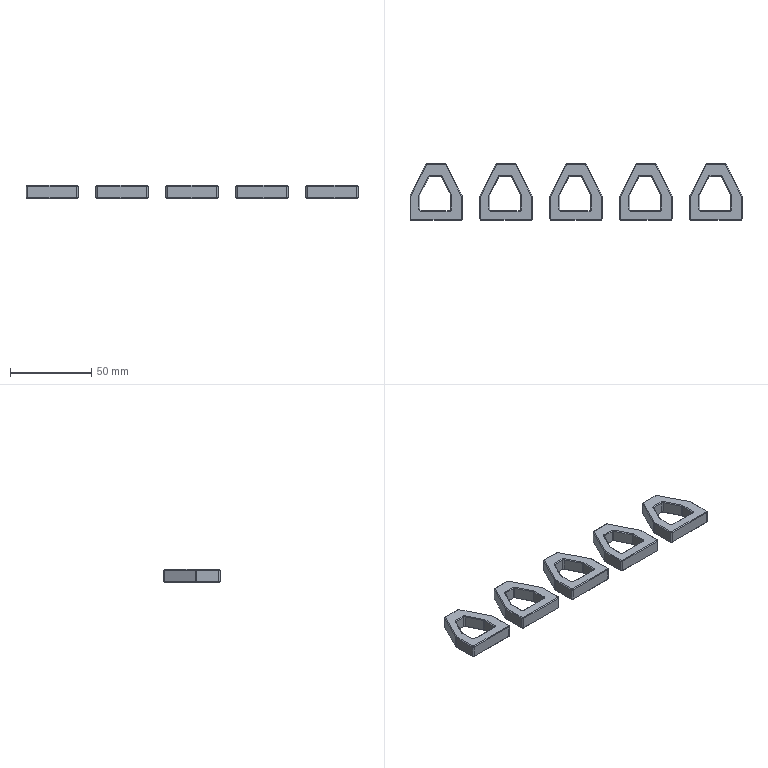NC program | NX | posted with a generic post | part box 204 x 35 x 8 mm
Lines 19 to 965 of 15564:
(ZLEVEL_PROFILE_COPY_1 , TOOL : D10)
N36 T15 M6
N38 G54
N40 G17 G0 G90 X4.326 Y-1.972 S9500 M3
N42 G43 Z30. H15
N44 Z1.5
N46 G94 G1 X1.14 Y4.4 Z1.127 F1000.
N48 X-0.14 Z1.06
N50 X-3.9 Y-3.12 Z0.619
N52 Y-6.4 Z0.447
N54 X4.9 Z-0.014
N56 Y-3.12 Z-0.186
N58 X1.14 Y4.4 Z-0.627
N60 X-0.14 Z-0.694
N62 X-2.753 Y-0.827 Z-1.
N64 X-3.9 Y-3.12 F3500.
N66 Y-6.4
N68 X4.9
N70 Y-3.12
N72 X1.14 Y4.4
N74 X-0.14
N76 X-2.753 Y-0.827
N78 X-3.9 Y-3.12 Z-1.077
N80 Y-6.4 Z-1.175
N82 X4.9 Z-1.438
N84 Y-3.12 Z-1.536
N86 X1.14 Y4.4 Z-1.787
N88 X-0.14 Z-1.825
N90 X-2.753 Y-0.827 Z-2.
N92 X-3.9 Y-3.12 Z-2.077
N94 Y-6.4 Z-2.175
N96 X4.9 Z-2.438
N98 Y-3.12 Z-2.536
N100 X1.14 Y4.4 Z-2.787
N102 X-0.14 Z-2.825
N104 X-2.753 Y-0.827 Z-3.
N106 X-3.9 Y-3.12 Z-3.077
N108 Y-6.4 Z-3.175
N110 X4.9 Z-3.438
N112 Y-3.12 Z-3.536
N114 X1.14 Y4.4 Z-3.787
N116 X-0.14 Z-3.825
N118 X-2.753 Y-0.827 Z-4.
N120 X-3.9 Y-3.12 Z-4.077
N122 Y-6.4 Z-4.175
N124 X4.9 Z-4.438
N126 Y-3.12 Z-4.536
N128 X1.14 Y4.4 Z-4.787
N130 X-0.14 Z-4.825
N132 X-2.753 Y-0.827 Z-5.
N134 X-3.9 Y-3.12 Z-5.077
N136 Y-6.4 Z-5.175
N138 X4.9 Z-5.438
N140 Y-3.12 Z-5.536
N142 X1.14 Y4.4 Z-5.787
N144 X-0.14 Z-5.825
N146 X-2.753 Y-0.827 Z-6.
N148 X-3.9 Y-3.12 Z-6.077
N150 Y-6.4 Z-6.175
N152 X4.9 Z-6.438
N154 Y-3.12 Z-6.536
N156 X1.14 Y4.4 Z-6.787
N158 X-0.14 Z-6.825
N160 X-2.753 Y-0.827 Z-7.
N162 X-3.9 Y-3.12 Z-7.077
N164 Y-6.4 Z-7.175
N166 X4.9 Z-7.438
N168 Y-3.12 Z-7.536
N170 X1.14 Y4.4 Z-7.787
N172 X-0.14 Z-7.825
N174 X-2.753 Y-0.827 Z-8.
N176 X-3.9 Y-3.12
N178 Y-6.4
N180 X4.9
N182 Y-3.12
N184 X1.14 Y4.4
N186 X-0.14
N188 X-2.753 Y-0.827
N190 Z-6.5
N192 G0 Z53.
N194 X-46.504 Y-6.4
N196 Z1.5
N198 G1 X-38.1 Z1.06 F1000.
N200 Y-3.12 Z0.888
N202 X-41.86 Y4.4 Z0.447
N204 X-43.14 Z0.38
N206 X-46.9 Y-3.12 Z-0.061
N208 Y-6.4 Z-0.233
N210 X-38.1 Z-0.694
N212 Y-3.12 Z-0.866
N214 X-39.247 Y-0.827 Z-1.
N216 X-41.86 Y4.4 F3500.
N218 X-43.14
N220 X-46.9 Y-3.12
N222 Y-6.4
N224 X-38.1
N226 Y-3.12
N228 X-39.247 Y-0.827
N230 X-41.86 Y4.4 Z-1.175
N232 X-43.14 Z-1.213
N234 X-46.9 Y-3.12 Z-1.464
N236 Y-6.4 Z-1.562
N238 X-38.1 Z-1.825
N240 Y-3.12 Z-1.923
N242 X-39.247 Y-0.827 Z-2.
N244 X-41.86 Y4.4 Z-2.175
N246 X-43.14 Z-2.213
N248 X-46.9 Y-3.12 Z-2.464
N250 Y-6.4 Z-2.562
N252 X-38.1 Z-2.825
N254 Y-3.12 Z-2.923
N256 X-39.247 Y-0.827 Z-3.
N258 X-41.86 Y4.4 Z-3.175
N260 X-43.14 Z-3.213
N262 X-46.9 Y-3.12 Z-3.464
N264 Y-6.4 Z-3.562
N266 X-38.1 Z-3.825
N268 Y-3.12 Z-3.923
N270 X-39.247 Y-0.827 Z-4.
N272 X-41.86 Y4.4 Z-4.175
N274 X-43.14 Z-4.213
N276 X-46.9 Y-3.12 Z-4.464
N278 Y-6.4 Z-4.562
N280 X-38.1 Z-4.825
N282 Y-3.12 Z-4.923
N284 X-39.247 Y-0.827 Z-5.
N286 X-41.86 Y4.4 Z-5.175
N288 X-43.14 Z-5.213
N290 X-46.9 Y-3.12 Z-5.464
N292 Y-6.4 Z-5.562
N294 X-38.1 Z-5.825
N296 Y-3.12 Z-5.923
N298 X-39.247 Y-0.827 Z-6.
N300 X-41.86 Y4.4 Z-6.175
N302 X-43.14 Z-6.213
N304 X-46.9 Y-3.12 Z-6.464
N306 Y-6.4 Z-6.562
N308 X-38.1 Z-6.825
N310 Y-3.12 Z-6.923
N312 X-39.247 Y-0.827 Z-7.
N314 X-41.86 Y4.4 Z-7.175
N316 X-43.14 Z-7.213
N318 X-46.9 Y-3.12 Z-7.464
N320 Y-6.4 Z-7.562
N322 X-38.1 Z-7.825
N324 Y-3.12 Z-7.923
N326 X-39.247 Y-0.827 Z-8.
N328 X-41.86 Y4.4
N330 X-43.14
N332 X-46.9 Y-3.12
N334 Y-6.4
N336 X-38.1
N338 Y-3.12
N340 X-39.247 Y-0.827
N342 Z-6.5
N344 G0 Z53.
N346 X-81.674 Y-1.972
N348 Z1.5
N350 G1 X-84.86 Y4.4 Z1.127 F1000.
N352 X-86.14 Z1.06
N354 X-89.9 Y-3.12 Z0.619
N356 Y-6.4 Z0.447
N358 X-81.1 Z-0.014
N360 Y-3.12 Z-0.186
N362 X-84.86 Y4.4 Z-0.627
N364 X-86.14 Z-0.694
N366 X-88.753 Y-0.827 Z-1.
N368 X-89.9 Y-3.12 F3500.
N370 Y-6.4
N372 X-81.1
N374 Y-3.12
N376 X-84.86 Y4.4
N378 X-86.14
N380 X-88.753 Y-0.827
N382 X-89.9 Y-3.12 Z-1.077
N384 Y-6.4 Z-1.175
N386 X-81.1 Z-1.438
N388 Y-3.12 Z-1.536
N390 X-84.86 Y4.4 Z-1.787
N392 X-86.14 Z-1.825
N394 X-88.753 Y-0.827 Z-2.
N396 X-89.9 Y-3.12 Z-2.077
N398 Y-6.4 Z-2.175
N400 X-81.1 Z-2.438
N402 Y-3.12 Z-2.536
N404 X-84.86 Y4.4 Z-2.787
N406 X-86.14 Z-2.825
N408 X-88.753 Y-0.827 Z-3.
N410 X-89.9 Y-3.12 Z-3.077
N412 Y-6.4 Z-3.175
N414 X-81.1 Z-3.438
N416 Y-3.12 Z-3.536
N418 X-84.86 Y4.4 Z-3.787
N420 X-86.14 Z-3.825
N422 X-88.753 Y-0.827 Z-4.
N424 X-89.9 Y-3.12 Z-4.077
N426 Y-6.4 Z-4.175
N428 X-81.1 Z-4.438
N430 Y-3.12 Z-4.536
N432 X-84.86 Y4.4 Z-4.787
N434 X-86.14 Z-4.825
N436 X-88.753 Y-0.827 Z-5.
N438 X-89.9 Y-3.12 Z-5.077
N440 Y-6.4 Z-5.175
N442 X-81.1 Z-5.438
N444 Y-3.12 Z-5.536
N446 X-84.86 Y4.4 Z-5.787
N448 X-86.14 Z-5.825
N450 X-88.753 Y-0.827 Z-6.
N452 X-89.9 Y-3.12 Z-6.077
N454 Y-6.4 Z-6.175
N456 X-81.1 Z-6.438
N458 Y-3.12 Z-6.536
N460 X-84.86 Y4.4 Z-6.787
N462 X-86.14 Z-6.825
N464 X-88.753 Y-0.827 Z-7.
N466 X-89.9 Y-3.12 Z-7.077
N468 Y-6.4 Z-7.175
N470 X-81.1 Z-7.438
N472 Y-3.12 Z-7.536
N474 X-84.86 Y4.4 Z-7.787
N476 X-86.14 Z-7.825
N478 X-88.753 Y-0.827 Z-8.
N480 X-89.9 Y-3.12
N482 Y-6.4
N484 X-81.1
N486 Y-3.12
N488 X-84.86 Y4.4
N490 X-86.14
N492 X-88.753 Y-0.827
N494 Z-6.5
N496 G0 Z53.
N498 X82.496 Y-6.4
N500 Z1.5
N502 G1 X90.9 Z1.06 F1000.
N504 Y-3.12 Z0.888
N506 X87.14 Y4.4 Z0.447
N508 X85.86 Z0.38
N510 X82.1 Y-3.12 Z-0.061
N512 Y-6.4 Z-0.233
N514 X90.9 Z-0.694
N516 Y-3.12 Z-0.866
N518 X89.753 Y-0.827 Z-1.
N520 X87.14 Y4.4 F3500.
N522 X85.86
N524 X82.1 Y-3.12
N526 Y-6.4
N528 X90.9
N530 Y-3.12
N532 X89.753 Y-0.827
N534 X87.14 Y4.4 Z-1.175
N536 X85.86 Z-1.213
N538 X82.1 Y-3.12 Z-1.464
N540 Y-6.4 Z-1.562
N542 X90.9 Z-1.825
N544 Y-3.12 Z-1.923
N546 X89.753 Y-0.827 Z-2.
N548 X87.14 Y4.4 Z-2.175
N550 X85.86 Z-2.213
N552 X82.1 Y-3.12 Z-2.464
N554 Y-6.4 Z-2.562
N556 X90.9 Z-2.825
N558 Y-3.12 Z-2.923
N560 X89.753 Y-0.827 Z-3.
N562 X87.14 Y4.4 Z-3.175
N564 X85.86 Z-3.213
N566 X82.1 Y-3.12 Z-3.464
N568 Y-6.4 Z-3.562
N570 X90.9 Z-3.825
N572 Y-3.12 Z-3.923
N574 X89.753 Y-0.827 Z-4.
N576 X87.14 Y4.4 Z-4.175
N578 X85.86 Z-4.213
N580 X82.1 Y-3.12 Z-4.464
N582 Y-6.4 Z-4.562
N584 X90.9 Z-4.825
N586 Y-3.12 Z-4.923
N588 X89.753 Y-0.827 Z-5.
N590 X87.14 Y4.4 Z-5.175
N592 X85.86 Z-5.213
N594 X82.1 Y-3.12 Z-5.464
N596 Y-6.4 Z-5.562
N598 X90.9 Z-5.825
N600 Y-3.12 Z-5.923
N602 X89.753 Y-0.827 Z-6.
N604 X87.14 Y4.4 Z-6.175
N606 X85.86 Z-6.213
N608 X82.1 Y-3.12 Z-6.464
N610 Y-6.4 Z-6.562
N612 X90.9 Z-6.825
N614 Y-3.12 Z-6.923
N616 X89.753 Y-0.827 Z-7.
N618 X87.14 Y4.4 Z-7.175
N620 X85.86 Z-7.213
N622 X82.1 Y-3.12 Z-7.464
N624 Y-6.4 Z-7.562
N626 X90.9 Z-7.825
N628 Y-3.12 Z-7.923
N630 X89.753 Y-0.827 Z-8.
N632 X87.14 Y4.4
N634 X85.86
N636 X82.1 Y-3.12
N638 Y-6.4
N640 X90.9
N642 Y-3.12
N644 X89.753 Y-0.827
N646 Z-6.5
N648 G0 Z53.
N650 X39.496 Y-6.4
N652 Z1.5
N654 G1 X47.9 Z1.06 F1000.
N656 Y-3.12 Z0.888
N658 X44.14 Y4.4 Z0.447
N660 X42.86 Z0.38
N662 X39.1 Y-3.12 Z-0.061
N664 Y-6.4 Z-0.233
N666 X47.9 Z-0.694
N668 Y-3.12 Z-0.866
N670 X46.753 Y-0.827 Z-1.
N672 X44.14 Y4.4 F3500.
N674 X42.86
N676 X39.1 Y-3.12
N678 Y-6.4
N680 X47.9
N682 Y-3.12
N684 X46.753 Y-0.827
N686 X44.14 Y4.4 Z-1.175
N688 X42.86 Z-1.213
N690 X39.1 Y-3.12 Z-1.464
N692 Y-6.4 Z-1.562
N694 X47.9 Z-1.825
N696 Y-3.12 Z-1.923
N698 X46.753 Y-0.827 Z-2.
N700 X44.14 Y4.4 Z-2.175
N702 X42.86 Z-2.213
N704 X39.1 Y-3.12 Z-2.464
N706 Y-6.4 Z-2.562
N708 X47.9 Z-2.825
N710 Y-3.12 Z-2.923
N712 X46.753 Y-0.827 Z-3.
N714 X44.14 Y4.4 Z-3.175
N716 X42.86 Z-3.213
N718 X39.1 Y-3.12 Z-3.464
N720 Y-6.4 Z-3.562
N722 X47.9 Z-3.825
N724 Y-3.12 Z-3.923
N726 X46.753 Y-0.827 Z-4.
N728 X44.14 Y4.4 Z-4.175
N730 X42.86 Z-4.213
N732 X39.1 Y-3.12 Z-4.464
N734 Y-6.4 Z-4.562
N736 X47.9 Z-4.825
N738 Y-3.12 Z-4.923
N740 X46.753 Y-0.827 Z-5.
N742 X44.14 Y4.4 Z-5.175
N744 X42.86 Z-5.213
N746 X39.1 Y-3.12 Z-5.464
N748 Y-6.4 Z-5.562
N750 X47.9 Z-5.825
N752 Y-3.12 Z-5.923
N754 X46.753 Y-0.827 Z-6.
N756 X44.14 Y4.4 Z-6.175
N758 X42.86 Z-6.213
N760 X39.1 Y-3.12 Z-6.464
N762 Y-6.4 Z-6.562
N764 X47.9 Z-6.825
N766 Y-3.12 Z-6.923
N768 X46.753 Y-0.827 Z-7.
N770 X44.14 Y4.4 Z-7.175
N772 X42.86 Z-7.213
N774 X39.1 Y-3.12 Z-7.464
N776 Y-6.4 Z-7.562
N778 X47.9 Z-7.825
N780 Y-3.12 Z-7.923
N782 X46.753 Y-0.827 Z-8.
N784 X44.14 Y4.4
N786 X42.86
N788 X39.1 Y-3.12
N790 Y-6.4
N792 X47.9
N794 Y-3.12
N796 X46.753 Y-0.827
N798 Z-6.5
N800 G0 Z53.
N802 X60.548 Y5.808
N804 Z1.5
N806 G1 X63.727 Y-0.55 Z1.127 F1000.
N808 X64.1 Y-2.13 Z1.042
N810 Y-17.106 Z0.258
N812 X63.707 Y-18.737 Z0.17
N814 X62.887 Y-20.201 Z0.082
N816 X61.701 Y-21.387 Z-0.006
N818 X60.237 Y-22.207 Z-0.094
N820 X58.606 Y-22.6 Z-0.182
N822 X43. Z-1.
N824 X28. F3500.
N826 G2 X21.9 Y-16.5 R6.1
N828 G1 Y-2.736
N830 G2 X22.544 Y-0.008 R6.1
N832 G1 X32.162 Y19.228
N834 G2 X37.618 Y22.6 R6.1
N836 G1 X48.382
N838 G2 X53.838 Y19.228 R6.1
N840 G1 X63.456 Y-0.008
N842 G2 X64.1 Y-2.736 R6.1
N844 G1 Y-16.5
N846 G2 X58. Y-22.6 R6.1
N848 G1 X43.
N850 X28. Z-1.1
N852 X27.402 Y-22.571 Z-1.104
N854 X26.81 Y-22.483 Z-1.108
N856 X26.229 Y-22.337 Z-1.112
N858 X25.666 Y-22.136 Z-1.116
N860 X25.124 Y-21.88 Z-1.12
N862 X24.611 Y-21.572 Z-1.124
N864 X24.13 Y-21.215 Z-1.128
N866 X23.687 Y-20.813 Z-1.132
N868 X23.285 Y-20.37 Z-1.136
N870 X22.928 Y-19.889 Z-1.14
N872 X22.62 Y-19.376 Z-1.144
N874 X22.364 Y-18.834 Z-1.148
N876 X22.163 Y-18.271 Z-1.152
N878 X22.017 Y-17.69 Z-1.156
N880 X21.929 Y-17.098 Z-1.16
N882 X21.9 Y-16.5 Z-1.164
N884 Y-2.736 Z-1.256
N886 X21.918 Y-2.265 Z-1.259
N888 X21.973 Y-1.797 Z-1.263
N890 X22.063 Y-1.335 Z-1.266
N892 X22.189 Y-0.88 Z-1.269
N894 X22.35 Y-0.437 Z-1.272
N896 X22.544 Y-0.008 Z-1.275
N898 X32.162 Y19.228 Z-1.419
N900 X32.437 Y19.719 Z-1.423
N902 X32.755 Y20.183 Z-1.426
N904 X33.115 Y20.615 Z-1.43
N906 X33.513 Y21.012 Z-1.434
N908 X33.947 Y21.371 Z-1.438
N910 X34.411 Y21.689 Z-1.441
N912 X34.903 Y21.962 Z-1.445
N914 X35.418 Y22.189 Z-1.449
N916 X35.951 Y22.368 Z-1.453
N918 X36.499 Y22.496 Z-1.457
N920 X37.056 Y22.574 Z-1.46
N922 X37.618 Y22.6 Z-1.464
N924 X48.382 Z-1.536
N926 X48.944 Y22.574 Z-1.54
N928 X49.501 Y22.496 Z-1.543
N930 X50.049 Y22.368 Z-1.547
N932 X50.582 Y22.189 Z-1.551
N934 X51.097 Y21.962 Z-1.555
N936 X51.589 Y21.689 Z-1.559
N938 X52.053 Y21.371 Z-1.562
N940 X52.487 Y21.012 Z-1.566
N942 X52.885 Y20.615 Z-1.57
N944 X53.245 Y20.183 Z-1.574
N946 X53.563 Y19.719 Z-1.577
N948 X53.838 Y19.228 Z-1.581
N950 X63.456 Y-0.008 Z-1.725
N952 X63.65 Y-0.437 Z-1.728
N954 X63.811 Y-0.88 Z-1.731
N956 X63.937 Y-1.335 Z-1.734
N958 X64.027 Y-1.797 Z-1.737
N960 X64.082 Y-2.265 Z-1.741
N962 X64.1 Y-2.736 Z-1.744
N964 Y-16.5 Z-1.836
N966 X64.071 Y-17.098 Z-1.84
N968 X63.983 Y-17.69 Z-1.844
N970 X63.837 Y-18.271 Z-1.848
N972 X63.636 Y-18.834 Z-1.852
N974 X63.38 Y-19.376 Z-1.856
N976 X63.072 Y-19.889 Z-1.86
N978 X62.715 Y-20.37 Z-1.864
N980 X62.313 Y-20.813 Z-1.868
N982 X61.87 Y-21.215 Z-1.872
N984 X61.389 Y-21.572 Z-1.876
N986 X60.876 Y-21.88 Z-1.88
N988 X60.334 Y-22.136 Z-1.884
N990 X59.771 Y-22.337 Z-1.888
N992 X59.19 Y-22.483 Z-1.892
N994 X58.598 Y-22.571 Z-1.896
N996 X58. Y-22.6 Z-1.9
N998 X43. Z-2.
N1000 X28. Z-2.1
N1002 X27.402 Y-22.571 Z-2.104
N1004 X26.81 Y-22.483 Z-2.108
N1006 X26.229 Y-22.337 Z-2.112
N1008 X25.666 Y-22.136 Z-2.116
N1010 X25.124 Y-21.88 Z-2.12
N1012 X24.611 Y-21.572 Z-2.124
N1014 X24.13 Y-21.215 Z-2.128
N1016 X23.687 Y-20.813 Z-2.132
N1018 X23.285 Y-20.37 Z-2.136
N1020 X22.928 Y-19.889 Z-2.14
N1022 X22.62 Y-19.376 Z-2.144
N1024 X22.364 Y-18.834 Z-2.148
N1026 X22.163 Y-18.271 Z-2.152
N1028 X22.017 Y-17.69 Z-2.156
N1030 X21.929 Y-17.098 Z-2.16
N1032 X21.9 Y-16.5 Z-2.164
N1034 Y-2.736 Z-2.256
N1036 X21.918 Y-2.265 Z-2.259
N1038 X21.973 Y-1.797 Z-2.263
N1040 X22.063 Y-1.335 Z-2.266
N1042 X22.189 Y-0.88 Z-2.269
N1044 X22.35 Y-0.437 Z-2.272
N1046 X22.544 Y-0.008 Z-2.275
N1048 X32.162 Y19.228 Z-2.419
N1050 X32.437 Y19.719 Z-2.423
N1052 X32.755 Y20.183 Z-2.426
N1054 X33.115 Y20.615 Z-2.43
N1056 X33.513 Y21.012 Z-2.434
N1058 X33.947 Y21.371 Z-2.438
N1060 X34.411 Y21.689 Z-2.441
N1062 X34.903 Y21.962 Z-2.445
N1064 X35.418 Y22.189 Z-2.449
N1066 X35.951 Y22.368 Z-2.453
N1068 X36.499 Y22.496 Z-2.457
N1070 X37.056 Y22.574 Z-2.46
N1072 X37.618 Y22.6 Z-2.464
N1074 X48.382 Z-2.536
N1076 X48.944 Y22.574 Z-2.54
N1078 X49.501 Y22.496 Z-2.543
N1080 X50.049 Y22.368 Z-2.547
N1082 X50.582 Y22.189 Z-2.551
N1084 X51.097 Y21.962 Z-2.555
N1086 X51.589 Y21.689 Z-2.559
N1088 X52.053 Y21.371 Z-2.562
N1090 X52.487 Y21.012 Z-2.566
N1092 X52.885 Y20.615 Z-2.57
N1094 X53.245 Y20.183 Z-2.574
N1096 X53.563 Y19.719 Z-2.577
N1098 X53.838 Y19.228 Z-2.581
N1100 X63.456 Y-0.008 Z-2.725
N1102 X63.65 Y-0.437 Z-2.728
N1104 X63.811 Y-0.88 Z-2.731
N1106 X63.937 Y-1.335 Z-2.734
N1108 X64.027 Y-1.797 Z-2.737
N1110 X64.082 Y-2.265 Z-2.741
N1112 X64.1 Y-2.736 Z-2.744
N1114 Y-16.5 Z-2.836
N1116 X64.071 Y-17.098 Z-2.84
N1118 X63.983 Y-17.69 Z-2.844
N1120 X63.837 Y-18.271 Z-2.848
N1122 X63.636 Y-18.834 Z-2.852
N1124 X63.38 Y-19.376 Z-2.856
N1126 X63.072 Y-19.889 Z-2.86
N1128 X62.715 Y-20.37 Z-2.864
N1130 X62.313 Y-20.813 Z-2.868
N1132 X61.87 Y-21.215 Z-2.872
N1134 X61.389 Y-21.572 Z-2.876
N1136 X60.876 Y-21.88 Z-2.88
N1138 X60.334 Y-22.136 Z-2.884
N1140 X59.771 Y-22.337 Z-2.888
N1142 X59.19 Y-22.483 Z-2.892
N1144 X58.598 Y-22.571 Z-2.896
N1146 X58. Y-22.6 Z-2.9
N1148 X43. Z-3.
N1150 X28. Z-3.1
N1152 X27.402 Y-22.571 Z-3.104
N1154 X26.81 Y-22.483 Z-3.108
N1156 X26.229 Y-22.337 Z-3.112
N1158 X25.666 Y-22.136 Z-3.116
N1160 X25.124 Y-21.88 Z-3.12
N1162 X24.611 Y-21.572 Z-3.124
N1164 X24.13 Y-21.215 Z-3.128
N1166 X23.687 Y-20.813 Z-3.132
N1168 X23.285 Y-20.37 Z-3.136
N1170 X22.928 Y-19.889 Z-3.14
N1172 X22.62 Y-19.376 Z-3.144
N1174 X22.364 Y-18.834 Z-3.148
N1176 X22.163 Y-18.271 Z-3.152
N1178 X22.017 Y-17.69 Z-3.156
N1180 X21.929 Y-17.098 Z-3.16
N1182 X21.9 Y-16.5 Z-3.164
N1184 Y-2.736 Z-3.256
N1186 X21.918 Y-2.265 Z-3.259
N1188 X21.973 Y-1.797 Z-3.263
N1190 X22.063 Y-1.335 Z-3.266
N1192 X22.189 Y-0.88 Z-3.269
N1194 X22.35 Y-0.437 Z-3.272
N1196 X22.544 Y-0.008 Z-3.275
N1198 X32.162 Y19.228 Z-3.419
N1200 X32.437 Y19.719 Z-3.423
N1202 X32.755 Y20.183 Z-3.426
N1204 X33.115 Y20.615 Z-3.43
N1206 X33.513 Y21.012 Z-3.434
N1208 X33.947 Y21.371 Z-3.438
N1210 X34.411 Y21.689 Z-3.441
N1212 X34.903 Y21.962 Z-3.445
N1214 X35.418 Y22.189 Z-3.449
N1216 X35.951 Y22.368 Z-3.453
N1218 X36.499 Y22.496 Z-3.457
N1220 X37.056 Y22.574 Z-3.46
N1222 X37.618 Y22.6 Z-3.464
N1224 X48.382 Z-3.536
N1226 X48.944 Y22.574 Z-3.54
N1228 X49.501 Y22.496 Z-3.543
N1230 X50.049 Y22.368 Z-3.547
N1232 X50.582 Y22.189 Z-3.551
N1234 X51.097 Y21.962 Z-3.555
N1236 X51.589 Y21.689 Z-3.559
N1238 X52.053 Y21.371 Z-3.562
N1240 X52.487 Y21.012 Z-3.566
N1242 X52.885 Y20.615 Z-3.57
N1244 X53.245 Y20.183 Z-3.574
N1246 X53.563 Y19.719 Z-3.577
N1248 X53.838 Y19.228 Z-3.581
N1250 X63.456 Y-0.008 Z-3.725
N1252 X63.65 Y-0.437 Z-3.728
N1254 X63.811 Y-0.88 Z-3.731
N1256 X63.937 Y-1.335 Z-3.734
N1258 X64.027 Y-1.797 Z-3.737
N1260 X64.082 Y-2.265 Z-3.741
N1262 X64.1 Y-2.736 Z-3.744
N1264 Y-16.5 Z-3.836
N1266 X64.071 Y-17.098 Z-3.84
N1268 X63.983 Y-17.69 Z-3.844
N1270 X63.837 Y-18.271 Z-3.848
N1272 X63.636 Y-18.834 Z-3.852
N1274 X63.38 Y-19.376 Z-3.856
N1276 X63.072 Y-19.889 Z-3.86
N1278 X62.715 Y-20.37 Z-3.864
N1280 X62.313 Y-20.813 Z-3.868
N1282 X61.87 Y-21.215 Z-3.872
N1284 X61.389 Y-21.572 Z-3.876
N1286 X60.876 Y-21.88 Z-3.88
N1288 X60.334 Y-22.136 Z-3.884
N1290 X59.771 Y-22.337 Z-3.888
N1292 X59.19 Y-22.483 Z-3.892
N1294 X58.598 Y-22.571 Z-3.896
N1296 X58. Y-22.6 Z-3.9
N1298 X43. Z-4.
N1300 X28. Z-4.1
N1302 X27.402 Y-22.571 Z-4.104
N1304 X26.81 Y-22.483 Z-4.108
N1306 X26.229 Y-22.337 Z-4.112
N1308 X25.666 Y-22.136 Z-4.116
N1310 X25.124 Y-21.88 Z-4.12
N1312 X24.611 Y-21.572 Z-4.124
N1314 X24.13 Y-21.215 Z-4.128
N1316 X23.687 Y-20.813 Z-4.132
N1318 X23.285 Y-20.37 Z-4.136
N1320 X22.928 Y-19.889 Z-4.14
N1322 X22.62 Y-19.376 Z-4.144
N1324 X22.364 Y-18.834 Z-4.148
N1326 X22.163 Y-18.271 Z-4.152
N1328 X22.017 Y-17.69 Z-4.156
N1330 X21.929 Y-17.098 Z-4.16
N1332 X21.9 Y-16.5 Z-4.164
N1334 Y-2.736 Z-4.256
N1336 X21.918 Y-2.265 Z-4.259
N1338 X21.973 Y-1.797 Z-4.263
N1340 X22.063 Y-1.335 Z-4.266
N1342 X22.189 Y-0.88 Z-4.269
N1344 X22.35 Y-0.437 Z-4.272
N1346 X22.544 Y-0.008 Z-4.275
N1348 X32.162 Y19.228 Z-4.419
N1350 X32.437 Y19.719 Z-4.423
N1352 X32.755 Y20.183 Z-4.426
N1354 X33.115 Y20.615 Z-4.43
N1356 X33.513 Y21.012 Z-4.434
N1358 X33.947 Y21.371 Z-4.438
N1360 X34.411 Y21.689 Z-4.441
N1362 X34.903 Y21.962 Z-4.445
N1364 X35.418 Y22.189 Z-4.449
N1366 X35.951 Y22.368 Z-4.453
N1368 X36.499 Y22.496 Z-4.457
N1370 X37.056 Y22.574 Z-4.46
N1372 X37.618 Y22.6 Z-4.464
N1374 X48.382 Z-4.536
N1376 X48.944 Y22.574 Z-4.54
N1378 X49.501 Y22.496 Z-4.543
N1380 X50.049 Y22.368 Z-4.547
N1382 X50.582 Y22.189 Z-4.551
N1384 X51.097 Y21.962 Z-4.555
N1386 X51.589 Y21.689 Z-4.559
N1388 X52.053 Y21.371 Z-4.562
N1390 X52.487 Y21.012 Z-4.566
N1392 X52.885 Y20.615 Z-4.57
N1394 X53.245 Y20.183 Z-4.574
N1396 X53.563 Y19.719 Z-4.577
N1398 X53.838 Y19.228 Z-4.581
N1400 X63.456 Y-0.008 Z-4.725
N1402 X63.65 Y-0.437 Z-4.728
N1404 X63.811 Y-0.88 Z-4.731
N1406 X63.937 Y-1.335 Z-4.734
N1408 X64.027 Y-1.797 Z-4.737
N1410 X64.082 Y-2.265 Z-4.741
N1412 X64.1 Y-2.736 Z-4.744
N1414 Y-16.5 Z-4.836
N1416 X64.071 Y-17.098 Z-4.84
N1418 X63.983 Y-17.69 Z-4.844
N1420 X63.837 Y-18.271 Z-4.848
N1422 X63.636 Y-18.834 Z-4.852
N1424 X63.38 Y-19.376 Z-4.856
N1426 X63.072 Y-19.889 Z-4.86
N1428 X62.715 Y-20.37 Z-4.864
N1430 X62.313 Y-20.813 Z-4.868
N1432 X61.87 Y-21.215 Z-4.872
N1434 X61.389 Y-21.572 Z-4.876
N1436 X60.876 Y-21.88 Z-4.88
N1438 X60.334 Y-22.136 Z-4.884
N1440 X59.771 Y-22.337 Z-4.888
N1442 X59.19 Y-22.483 Z-4.892
N1444 X58.598 Y-22.571 Z-4.896
N1446 X58. Y-22.6 Z-4.9
N1448 X43. Z-5.
N1450 X28. Z-5.1
N1452 X27.402 Y-22.571 Z-5.104
N1454 X26.81 Y-22.483 Z-5.108
N1456 X26.229 Y-22.337 Z-5.112
N1458 X25.666 Y-22.136 Z-5.116
N1460 X25.124 Y-21.88 Z-5.12
N1462 X24.611 Y-21.572 Z-5.124
N1464 X24.13 Y-21.215 Z-5.128
N1466 X23.687 Y-20.813 Z-5.132
N1468 X23.285 Y-20.37 Z-5.136
N1470 X22.928 Y-19.889 Z-5.14
N1472 X22.62 Y-19.376 Z-5.144
N1474 X22.364 Y-18.834 Z-5.148
N1476 X22.163 Y-18.271 Z-5.152
N1478 X22.017 Y-17.69 Z-5.156
N1480 X21.929 Y-17.098 Z-5.16
N1482 X21.9 Y-16.5 Z-5.164
N1484 Y-2.736 Z-5.256
N1486 X21.918 Y-2.265 Z-5.259
N1488 X21.973 Y-1.797 Z-5.263
N1490 X22.063 Y-1.335 Z-5.266
N1492 X22.189 Y-0.88 Z-5.269
N1494 X22.35 Y-0.437 Z-5.272
N1496 X22.544 Y-0.008 Z-5.275
N1498 X32.162 Y19.228 Z-5.419
N1500 X32.437 Y19.719 Z-5.423
N1502 X32.755 Y20.183 Z-5.426
N1504 X33.115 Y20.615 Z-5.43
N1506 X33.513 Y21.012 Z-5.434
N1508 X33.947 Y21.371 Z-5.438
N1510 X34.411 Y21.689 Z-5.441
N1512 X34.903 Y21.962 Z-5.445
N1514 X35.418 Y22.189 Z-5.449
N1516 X35.951 Y22.368 Z-5.453
N1518 X36.499 Y22.496 Z-5.457
N1520 X37.056 Y22.574 Z-5.46
N1522 X37.618 Y22.6 Z-5.464
N1524 X48.382 Z-5.536
N1526 X48.944 Y22.574 Z-5.54
N1528 X49.501 Y22.496 Z-5.543
N1530 X50.049 Y22.368 Z-5.547
N1532 X50.582 Y22.189 Z-5.551
N1534 X51.097 Y21.962 Z-5.555
N1536 X51.589 Y21.689 Z-5.559
N1538 X52.053 Y21.371 Z-5.562
N1540 X52.487 Y21.012 Z-5.566
N1542 X52.885 Y20.615 Z-5.57
N1544 X53.245 Y20.183 Z-5.574
N1546 X53.563 Y19.719 Z-5.577
N1548 X53.838 Y19.228 Z-5.581
N1550 X63.456 Y-0.008 Z-5.725
N1552 X63.65 Y-0.437 Z-5.728
N1554 X63.811 Y-0.88 Z-5.731
N1556 X63.937 Y-1.335 Z-5.734
N1558 X64.027 Y-1.797 Z-5.737
N1560 X64.082 Y-2.265 Z-5.741
N1562 X64.1 Y-2.736 Z-5.744
N1564 Y-16.5 Z-5.836
N1566 X64.071 Y-17.098 Z-5.84
N1568 X63.983 Y-17.69 Z-5.844
N1570 X63.837 Y-18.271 Z-5.848
N1572 X63.636 Y-18.834 Z-5.852
N1574 X63.38 Y-19.376 Z-5.856
N1576 X63.072 Y-19.889 Z-5.86
N1578 X62.715 Y-20.37 Z-5.864
N1580 X62.313 Y-20.813 Z-5.868
N1582 X61.87 Y-21.215 Z-5.872
N1584 X61.389 Y-21.572 Z-5.876
N1586 X60.876 Y-21.88 Z-5.88
N1588 X60.334 Y-22.136 Z-5.884
N1590 X59.771 Y-22.337 Z-5.888
N1592 X59.19 Y-22.483 Z-5.892
N1594 X58.598 Y-22.571 Z-5.896
N1596 X58. Y-22.6 Z-5.9
N1598 X43. Z-6.
N1600 X28. Z-6.1
N1602 X27.402 Y-22.571 Z-6.104
N1604 X26.81 Y-22.483 Z-6.108
N1606 X26.229 Y-22.337 Z-6.112
N1608 X25.666 Y-22.136 Z-6.116
N1610 X25.124 Y-21.88 Z-6.12
N1612 X24.611 Y-21.572 Z-6.124
N1614 X24.13 Y-21.215 Z-6.128
N1616 X23.687 Y-20.813 Z-6.132
N1618 X23.285 Y-20.37 Z-6.136
N1620 X22.928 Y-19.889 Z-6.14
N1622 X22.62 Y-19.376 Z-6.144
N1624 X22.364 Y-18.834 Z-6.148
N1626 X22.163 Y-18.271 Z-6.152
N1628 X22.017 Y-17.69 Z-6.156
N1630 X21.929 Y-17.098 Z-6.16
N1632 X21.9 Y-16.5 Z-6.164
N1634 Y-2.736 Z-6.256
N1636 X21.918 Y-2.265 Z-6.259
N1638 X21.973 Y-1.797 Z-6.263
N1640 X22.063 Y-1.335 Z-6.266
N1642 X22.189 Y-0.88 Z-6.269
N1644 X22.35 Y-0.437 Z-6.272
N1646 X22.544 Y-0.008 Z-6.275
N1648 X32.162 Y19.228 Z-6.419
N1650 X32.437 Y19.719 Z-6.423
N1652 X32.755 Y20.183 Z-6.426
N1654 X33.115 Y20.615 Z-6.43
N1656 X33.513 Y21.012 Z-6.434
N1658 X33.947 Y21.371 Z-6.438
N1660 X34.411 Y21.689 Z-6.441
N1662 X34.903 Y21.962 Z-6.445
N1664 X35.418 Y22.189 Z-6.449
N1666 X35.951 Y22.368 Z-6.453
N1668 X36.499 Y22.496 Z-6.457
N1670 X37.056 Y22.574 Z-6.46
N1672 X37.618 Y22.6 Z-6.464
N1674 X48.382 Z-6.536
N1676 X48.944 Y22.574 Z-6.54
N1678 X49.501 Y22.496 Z-6.543
N1680 X50.049 Y22.368 Z-6.547
N1682 X50.582 Y22.189 Z-6.551
N1684 X51.097 Y21.962 Z-6.555
N1686 X51.589 Y21.689 Z-6.559
N1688 X52.053 Y21.371 Z-6.562
N1690 X52.487 Y21.012 Z-6.566
N1692 X52.885 Y20.615 Z-6.57
N1694 X53.245 Y20.183 Z-6.574
N1696 X53.563 Y19.719 Z-6.577
N1698 X53.838 Y19.228 Z-6.581
N1700 X63.456 Y-0.008 Z-6.725
N1702 X63.65 Y-0.437 Z-6.728
N1704 X63.811 Y-0.88 Z-6.731
N1706 X63.937 Y-1.335 Z-6.734
N1708 X64.027 Y-1.797 Z-6.737
N1710 X64.082 Y-2.265 Z-6.741
N1712 X64.1 Y-2.736 Z-6.744
N1714 Y-16.5 Z-6.836
N1716 X64.071 Y-17.098 Z-6.84
N1718 X63.983 Y-17.69 Z-6.844
N1720 X63.837 Y-18.271 Z-6.848
N1722 X63.636 Y-18.834 Z-6.852
N1724 X63.38 Y-19.376 Z-6.856
N1726 X63.072 Y-19.889 Z-6.86
N1728 X62.715 Y-20.37 Z-6.864
N1730 X62.313 Y-20.813 Z-6.868
N1732 X61.87 Y-21.215 Z-6.872
N1734 X61.389 Y-21.572 Z-6.876
N1736 X60.876 Y-21.88 Z-6.88
N1738 X60.334 Y-22.136 Z-6.884
N1740 X59.771 Y-22.337 Z-6.888
N1742 X59.19 Y-22.483 Z-6.892
N1744 X58.598 Y-22.571 Z-6.896
N1746 X58. Y-22.6 Z-6.9
N1748 X43. Z-7.
N1750 X28. Z-7.1
N1752 X27.402 Y-22.571 Z-7.104
N1754 X26.81 Y-22.483 Z-7.108
N1756 X26.229 Y-22.337 Z-7.112
N1758 X25.666 Y-22.136 Z-7.116
N1760 X25.124 Y-21.88 Z-7.12
N1762 X24.611 Y-21.572 Z-7.124
N1764 X24.13 Y-21.215 Z-7.128
N1766 X23.687 Y-20.813 Z-7.132
N1768 X23.285 Y-20.37 Z-7.136
N1770 X22.928 Y-19.889 Z-7.14
N1772 X22.62 Y-19.376 Z-7.144
N1774 X22.364 Y-18.834 Z-7.148
N1776 X22.163 Y-18.271 Z-7.152
N1778 X22.017 Y-17.69 Z-7.156
N1780 X21.929 Y-17.098 Z-7.16
N1782 X21.9 Y-16.5 Z-7.164
N1784 Y-2.736 Z-7.256
N1786 X21.918 Y-2.265 Z-7.259
N1788 X21.973 Y-1.797 Z-7.263
N1790 X22.063 Y-1.335 Z-7.266
N1792 X22.189 Y-0.88 Z-7.269
N1794 X22.35 Y-0.437 Z-7.272
N1796 X22.544 Y-0.008 Z-7.275
N1798 X32.162 Y19.228 Z-7.419
N1800 X32.437 Y19.719 Z-7.423
N1802 X32.755 Y20.183 Z-7.426
N1804 X33.115 Y20.615 Z-7.43
N1806 X33.513 Y21.012 Z-7.434
N1808 X33.947 Y21.371 Z-7.438
N1810 X34.411 Y21.689 Z-7.441
N1812 X34.903 Y21.962 Z-7.445
N1814 X35.418 Y22.189 Z-7.449
N1816 X35.951 Y22.368 Z-7.453
N1818 X36.499 Y22.496 Z-7.457
N1820 X37.056 Y22.574 Z-7.46
N1822 X37.618 Y22.6 Z-7.464
N1824 X48.382 Z-7.536
N1826 X48.944 Y22.574 Z-7.54
N1828 X49.501 Y22.496 Z-7.543
N1830 X50.049 Y22.368 Z-7.547
N1832 X50.582 Y22.189 Z-7.551
N1834 X51.097 Y21.962 Z-7.555
N1836 X51.589 Y21.689 Z-7.559
N1838 X52.053 Y21.371 Z-7.562
N1840 X52.487 Y21.012 Z-7.566
N1842 X52.885 Y20.615 Z-7.57
N1844 X53.245 Y20.183 Z-7.574
N1846 X53.563 Y19.719 Z-7.577
N1848 X53.838 Y19.228 Z-7.581
N1850 X63.456 Y-0.008 Z-7.725
N1852 X63.65 Y-0.437 Z-7.728
N1854 X63.811 Y-0.88 Z-7.731
N1856 X63.937 Y-1.335 Z-7.734
N1858 X64.027 Y-1.797 Z-7.737
N1860 X64.082 Y-2.265 Z-7.741
N1862 X64.1 Y-2.736 Z-7.744
N1864 Y-16.5 Z-7.836
N1866 X64.071 Y-17.098 Z-7.84
N1868 X63.983 Y-17.69 Z-7.844
N1870 X63.837 Y-18.271 Z-7.848
N1872 X63.636 Y-18.834 Z-7.852
N1874 X63.38 Y-19.376 Z-7.856
N1876 X63.072 Y-19.889 Z-7.86
N1878 X62.715 Y-20.37 Z-7.864
N1880 X62.313 Y-20.813 Z-7.868
N1882 X61.87 Y-21.215 Z-7.872
N1884 X61.389 Y-21.572 Z-7.876
N1886 X60.876 Y-21.88 Z-7.88
N1888 X60.334 Y-22.136 Z-7.884
N1890 X59.771 Y-22.337 Z-7.888
N1892 X59.19 Y-22.483 Z-7.892
N1894 X58.598 Y-22.571 Z-7.896
N1896 X58. Y-22.6 Z-7.9
N1898 X43. Z-8.
N1900 X28.
N1902 G2 X21.9 Y-16.5 R6.1
N1904 G1 Y-2.736
N1906 G2 X22.544 Y-0.008 R6.1
N1908 G1 X32.162 Y19.228
N1910 G2 X37.618 Y22.6 R6.1
N1912 G1 X48.382
N1914 G2 X53.838 Y19.228 R6.1
N1916 G1 X63.456 Y-0.008
N1918 G2 X64.1 Y-2.736 R6.1
N1920 G1 Y-16.5
N1922 G2 X58. Y-22.6 R6.1